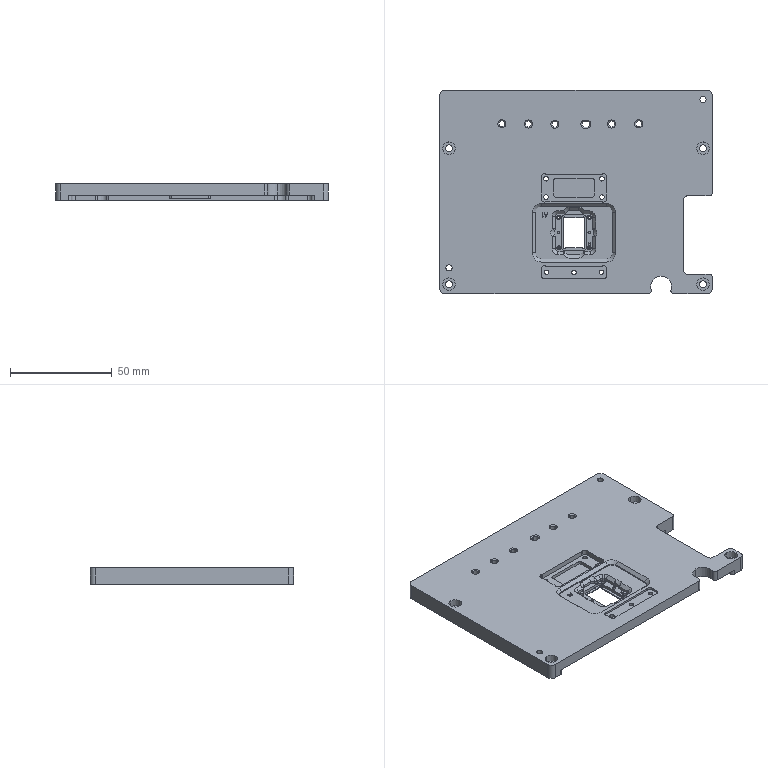NC program | NX | posted with a generic post | part box 134 x 100 x 8 mm
Lines 2719 to 3418 of 3418:
(CUTTERCOMP20 , TOOL : D1)
N5376 T20 M6
N5378 G54
N5380 G17 G0 G90 X0.695 Y-29.394 S9500 M3
N5382 G43 Z30. H20
N5384 Z-0.4
N5386 G94 G1 X0.839 Y-29.355 Z-0.408 F1000.
N5388 X1.143 Y-29.352 Z-0.424
N5390 X1.486 Y-29.45 Z-0.442
N5392 X1.783 Y-29.649 Z-0.461
N5394 X2.005 Y-29.928 Z-0.48
N5396 X2.119 Y-30.209 Z-0.496
N5398 X2.154 Y-30.578 Z-0.515
N5400 X2.07 Y-30.938 Z-0.535
N5402 X1.877 Y-31.254 Z-0.554
N5404 X1.594 Y-31.493 Z-0.573
N5406 X1.25 Y-31.629 Z-0.593
N5408 X1.049 Y-31.647 Z-0.603
N5410 X0.991 Z-0.606
N5412 X0.839 Y-31.645 Z-0.614
N5414 X0.441 Y-31.512 Z-0.636
N5416 X0.116 Y-31.246 Z-0.658
N5418 X-0.092 Y-30.881 Z-0.68
N5420 X-0.156 Y-30.466 Z-0.702
N5422 X-0.068 Y-30.056 Z-0.724
N5424 X0.084 Y-29.793 Z-0.74
N5426 X0.295 Y-29.583 Z-0.756
N5428 X0.552 Y-29.434 Z-0.771
N5430 X0.839 Y-29.355 Z-0.787
N5432 X1.143 Y-29.352 Z-0.803
N5434 X1.486 Y-29.45 Z-0.822
N5436 X1.783 Y-29.649 Z-0.84
N5438 X2.005 Y-29.928 Z-0.859
N5440 X2.119 Y-30.209 Z-0.875
N5442 X2.154 Y-30.578 Z-0.894
N5444 X2.07 Y-30.938 Z-0.914
N5446 X1.877 Y-31.254 Z-0.933
N5448 X1.594 Y-31.493 Z-0.953
N5450 X1.25 Y-31.629 Z-0.972
N5452 X1.098 Y-31.642 Z-0.98
N5454 G41 X1. Y-31.625 D20
N5456 X0.991
N5458 G2 X-0.125 Y-30.491 R1.125
N5460 X1. Y-31.625 R-1.125
N5462 G1 X0.928 Y-31.623 Z-0.981
N5464 X0.857 Y-31.616 Z-0.983
N5466 X0.786 Y-31.605 Z-0.984
N5468 X0.717 Y-31.589 Z-0.985
N5470 X0.648 Y-31.568 Z-0.986
N5472 X0.581 Y-31.544 Z-0.988
N5474 X0.515 Y-31.515 Z-0.989
N5476 X0.452 Y-31.482 Z-0.99
N5478 X0.39 Y-31.445 Z-0.991
N5480 X0.331 Y-31.405 Z-0.993
N5482 X0.275 Y-31.36 Z-0.994
N5484 X0.222 Y-31.313 Z-0.995
N5486 X0.172 Y-31.261 Z-0.996
N5488 X0.125 Y-31.207 Z-0.998
N5490 X0.082 Y-31.15 Z-0.999
N5492 X0.042 Y-31.09 Z-1.
N5494 X0.007 Y-31.028 Z-1.001
N5496 X-0.025 Y-30.964 Z-1.003
N5498 X-0.052 Y-30.898 Z-1.004
N5500 X-0.076 Y-30.83 Z-1.005
N5502 X-0.094 Y-30.761 Z-1.006
N5504 X-0.109 Y-30.691 Z-1.008
N5506 X-0.119 Y-30.62 Z-1.009
N5508 X-0.124 Y-30.548 Z-1.01
N5510 X-0.125 Y-30.477 Z-1.011
N5512 X-0.121 Y-30.405 Z-1.013
N5514 X-0.113 Y-30.334 Z-1.014
N5516 X-0.1 Y-30.264 Z-1.015
N5518 X-0.083 Y-30.194 Z-1.016
N5520 X-0.061 Y-30.126 Z-1.018
N5522 X-0.035 Y-30.059 Z-1.019
N5524 X-0.005 Y-29.994 Z-1.02
N5526 X0.029 Y-29.931 Z-1.021
N5528 X0.067 Y-29.871 Z-1.023
N5530 X0.109 Y-29.813 Z-1.024
N5532 X0.155 Y-29.758 Z-1.025
N5534 X0.204 Y-29.705 Z-1.026
N5536 X0.256 Y-29.656 Z-1.028
N5538 X0.311 Y-29.611 Z-1.029
N5540 X0.369 Y-29.569 Z-1.03
N5542 X0.43 Y-29.53 Z-1.031
N5544 X0.492 Y-29.496 Z-1.033
N5546 X0.557 Y-29.466 Z-1.034
N5548 X0.624 Y-29.44 Z-1.035
N5550 X0.692 Y-29.418 Z-1.036
N5552 X0.762 Y-29.401 Z-1.038
N5554 X0.832 Y-29.388 Z-1.039
N5556 X0.903 Y-29.379 Z-1.04
N5558 X0.975 Y-29.375 Z-1.041
N5560 X1.046 Y-29.376 Z-1.043
N5562 X1.118 Y-29.381 Z-1.044
N5564 X1.189 Y-29.391 Z-1.045
N5566 X1.259 Y-29.405 Z-1.046
N5568 X1.328 Y-29.424 Z-1.048
N5570 X1.396 Y-29.447 Z-1.049
N5572 X1.462 Y-29.474 Z-1.05
N5574 X1.526 Y-29.506 Z-1.051
N5576 X1.588 Y-29.541 Z-1.053
N5578 X1.648 Y-29.581 Z-1.054
N5580 X1.706 Y-29.623 Z-1.055
N5582 X1.76 Y-29.67 Z-1.056
N5584 X1.811 Y-29.72 Z-1.058
N5586 X1.859 Y-29.773 Z-1.059
N5588 X1.903 Y-29.83 Z-1.06
N5590 G2 X1. Y-31.625 R1.125
N5592 G1 X0.928 Y-31.623 Z-1.061
N5594 X0.857 Y-31.616 Z-1.063
N5596 X0.786 Y-31.605 Z-1.064
N5598 X0.717 Y-31.589 Z-1.065
N5600 X0.648 Y-31.568 Z-1.066
N5602 X0.581 Y-31.544 Z-1.068
N5604 X0.515 Y-31.515 Z-1.069
N5606 X0.452 Y-31.482 Z-1.07
N5608 X0.39 Y-31.445 Z-1.071
N5610 X0.331 Y-31.405 Z-1.073
N5612 X0.275 Y-31.36 Z-1.074
N5614 X0.222 Y-31.312 Z-1.075
N5616 X0.172 Y-31.261 Z-1.076
N5618 X0.125 Y-31.207 Z-1.078
N5620 X0.082 Y-31.15 Z-1.079
N5622 X0.042 Y-31.09 Z-1.08
N5624 X0.007 Y-31.028 Z-1.081
N5626 X-0.025 Y-30.964 Z-1.083
N5628 X-0.052 Y-30.898 Z-1.084
N5630 X-0.076 Y-30.83 Z-1.085
N5632 X-0.094 Y-30.761 Z-1.086
N5634 X-0.109 Y-30.691 Z-1.088
N5636 X-0.119 Y-30.62 Z-1.089
N5638 X-0.124 Y-30.548 Z-1.09
N5640 X-0.125 Y-30.477 Z-1.091
N5642 X-0.121 Y-30.405 Z-1.093
N5644 X-0.113 Y-30.334 Z-1.094
N5646 X-0.1 Y-30.264 Z-1.095
N5648 X-0.083 Y-30.194 Z-1.096
N5650 X-0.061 Y-30.126 Z-1.098
N5652 X-0.035 Y-30.059 Z-1.099
N5654 X-0.005 Y-29.994 Z-1.1
N5656 X0.029 Y-29.931 Z-1.101
N5658 X0.067 Y-29.871 Z-1.103
N5660 X0.109 Y-29.813 Z-1.104
N5662 X0.155 Y-29.758 Z-1.105
N5664 X0.204 Y-29.705 Z-1.106
N5666 X0.256 Y-29.656 Z-1.108
N5668 X0.311 Y-29.611 Z-1.109
N5670 X0.369 Y-29.569 Z-1.11
N5672 X0.43 Y-29.53 Z-1.111
N5674 X0.492 Y-29.496 Z-1.113
N5676 X0.557 Y-29.466 Z-1.114
N5678 X0.624 Y-29.439 Z-1.115
N5680 X0.692 Y-29.418 Z-1.116
N5682 X0.762 Y-29.401 Z-1.118
N5684 X0.832 Y-29.388 Z-1.119
N5686 X0.903 Y-29.379 Z-1.12
N5688 X0.975 Y-29.375 Z-1.121
N5690 X1.046 Y-29.376 Z-1.123
N5692 X1.118 Y-29.381 Z-1.124
N5694 X1.189 Y-29.391 Z-1.125
N5696 X1.259 Y-29.405 Z-1.126
N5698 X1.328 Y-29.424 Z-1.128
N5700 X1.396 Y-29.447 Z-1.129
N5702 X1.462 Y-29.474 Z-1.13
N5704 X1.526 Y-29.506 Z-1.131
N5706 X1.588 Y-29.541 Z-1.133
N5708 G2 X1. Y-31.625 R1.125
N5710 G1 X0.928 Y-31.623 Z-1.134
N5712 X0.857 Y-31.616 Z-1.135
N5714 X0.786 Y-31.605 Z-1.136
N5716 X0.717 Y-31.589 Z-1.138
N5718 X0.648 Y-31.569 Z-1.139
N5720 X0.581 Y-31.544 Z-1.14
N5722 X0.515 Y-31.515 Z-1.141
N5724 X0.452 Y-31.482 Z-1.143
N5726 X0.39 Y-31.445 Z-1.144
N5728 X0.331 Y-31.405 Z-1.145
N5730 X0.275 Y-31.36 Z-1.146
N5732 X0.222 Y-31.312 Z-1.148
N5734 X0.172 Y-31.261 Z-1.149
N5736 X0.125 Y-31.207 Z-1.15
N5738 X0.082 Y-31.15 Z-1.151
N5740 X0.042 Y-31.09 Z-1.153
N5742 X0.007 Y-31.028 Z-1.154
N5744 X-0.025 Y-30.964 Z-1.155
N5746 X-0.052 Y-30.898 Z-1.156
N5748 X-0.076 Y-30.83 Z-1.158
N5750 X-0.094 Y-30.761 Z-1.159
N5752 X-0.109 Y-30.691 Z-1.16
N5754 X-0.119 Y-30.62 Z-1.161
N5756 X-0.124 Y-30.548 Z-1.163
N5758 X-0.125 Y-30.477 Z-1.164
N5760 X-0.121 Y-30.405 Z-1.165
N5762 X-0.113 Y-30.334 Z-1.166
N5764 X-0.1 Y-30.264 Z-1.168
N5766 X-0.083 Y-30.194 Z-1.169
N5768 X-0.061 Y-30.126 Z-1.17
N5770 X-0.035 Y-30.059 Z-1.171
N5772 X-0.005 Y-29.994 Z-1.173
N5774 X0.029 Y-29.931 Z-1.174
N5776 X0.067 Y-29.871 Z-1.175
N5778 X0.109 Y-29.813 Z-1.176
N5780 X0.155 Y-29.758 Z-1.178
N5782 X0.204 Y-29.705 Z-1.179
N5784 X0.256 Y-29.656 Z-1.18
N5786 X0.311 Y-29.611 Z-1.181
N5788 X0.369 Y-29.568 Z-1.183
N5790 X0.43 Y-29.53 Z-1.184
N5792 X0.492 Y-29.496 Z-1.185
N5794 X0.557 Y-29.466 Z-1.186
N5796 X0.624 Y-29.439 Z-1.188
N5798 X0.692 Y-29.418 Z-1.189
N5800 X0.762 Y-29.401 Z-1.19
N5802 X0.832 Y-29.388 Z-1.191
N5804 X0.903 Y-29.379 Z-1.193
N5806 X0.975 Y-29.375 Z-1.194
N5808 X1.046 Y-29.376 Z-1.195
N5810 X1.118 Y-29.381 Z-1.196
N5812 X1.189 Y-29.391 Z-1.198
N5814 X1.259 Y-29.405 Z-1.199
N5816 X1.328 Y-29.424 Z-1.2
N5818 X1.396 Y-29.447 Z-1.201
N5820 X1.462 Y-29.474 Z-1.203
N5822 X1.526 Y-29.506 Z-1.204
N5824 X1.588 Y-29.541 Z-1.205
N5826 G2 X1. Y-31.625 R1.125
N5828 G1 X0.928 Y-31.623 Z-1.206
N5830 X0.857 Y-31.616 Z-1.208
N5832 X0.786 Y-31.605 Z-1.209
N5834 X0.717 Y-31.589 Z-1.21
N5836 X0.648 Y-31.569 Z-1.211
N5838 X0.581 Y-31.544 Z-1.213
N5840 X0.515 Y-31.515 Z-1.214
N5842 X0.452 Y-31.482 Z-1.215
N5844 X0.39 Y-31.445 Z-1.216
N5846 X0.331 Y-31.405 Z-1.218
N5848 X0.275 Y-31.36 Z-1.219
N5850 X0.222 Y-31.312 Z-1.22
N5852 X0.172 Y-31.261 Z-1.221
N5854 X0.125 Y-31.207 Z-1.223
N5856 X0.082 Y-31.15 Z-1.224
N5858 X0.042 Y-31.09 Z-1.225
N5860 X0.007 Y-31.028 Z-1.226
N5862 X-0.025 Y-30.964 Z-1.228
N5864 X-0.052 Y-30.898 Z-1.229
N5866 X-0.076 Y-30.83 Z-1.23
N5868 X-0.094 Y-30.761 Z-1.231
N5870 X-0.109 Y-30.691 Z-1.233
N5872 X-0.119 Y-30.62 Z-1.234
N5874 X-0.124 Y-30.548 Z-1.235
N5876 X-0.125 Y-30.477 Z-1.236
N5878 X-0.121 Y-30.405 Z-1.238
N5880 X-0.113 Y-30.334 Z-1.239
N5882 X-0.1 Y-30.264 Z-1.24
N5884 X-0.083 Y-30.194 Z-1.241
N5886 X-0.061 Y-30.126 Z-1.243
N5888 X-0.035 Y-30.059 Z-1.244
N5890 X-0.005 Y-29.994 Z-1.245
N5892 X0.029 Y-29.931 Z-1.246
N5894 X0.067 Y-29.871 Z-1.248
N5896 X0.109 Y-29.813 Z-1.249
N5898 X0.155 Y-29.758 Z-1.25
N5900 X0.204 Y-29.705 Z-1.251
N5902 X0.256 Y-29.656 Z-1.253
N5904 X0.311 Y-29.611 Z-1.254
N5906 X0.369 Y-29.568 Z-1.255
N5908 X0.43 Y-29.53 Z-1.256
N5910 X0.492 Y-29.496 Z-1.258
N5912 X0.557 Y-29.466 Z-1.259
N5914 X0.624 Y-29.439 Z-1.26
N5916 X0.692 Y-29.418 Z-1.261
N5918 X0.762 Y-29.401 Z-1.263
N5920 X0.832 Y-29.388 Z-1.264
N5922 X0.903 Y-29.379 Z-1.265
N5924 X0.975 Y-29.375 Z-1.266
N5926 X1.046 Y-29.376 Z-1.268
N5928 X1.118 Y-29.381 Z-1.269
N5930 X1.189 Y-29.391 Z-1.27
N5932 X1.259 Y-29.405 Z-1.271
N5934 X1.328 Y-29.424 Z-1.273
N5936 X1.396 Y-29.447 Z-1.274
N5938 X1.462 Y-29.474 Z-1.275
N5940 X1.526 Y-29.506 Z-1.276
N5942 X1.588 Y-29.541 Z-1.278
N5944 G2 X1. Y-31.625 R1.125
N5946 G1 X0.928 Y-31.623 Z-1.279
N5948 X0.857 Y-31.616 Z-1.28
N5950 X0.786 Y-31.605 Z-1.281
N5952 X0.717 Y-31.589 Z-1.283
N5954 X0.648 Y-31.568 Z-1.284
N5956 X0.581 Y-31.544 Z-1.285
N5958 X0.515 Y-31.515 Z-1.286
N5960 X0.452 Y-31.482 Z-1.288
N5962 X0.39 Y-31.445 Z-1.289
N5964 X0.331 Y-31.405 Z-1.29
N5966 X0.275 Y-31.36 Z-1.291
N5968 X0.222 Y-31.312 Z-1.293
N5970 X0.172 Y-31.261 Z-1.294
N5972 X0.125 Y-31.207 Z-1.295
N5974 X0.082 Y-31.15 Z-1.296
N5976 X0.042 Y-31.09 Z-1.298
N5978 X0.007 Y-31.028 Z-1.299
N5980 X-0.025 Y-30.964 Z-1.3
N5982 X-0.052 Y-30.898 Z-1.301
N5984 X-0.076 Y-30.83 Z-1.303
N5986 X-0.094 Y-30.761 Z-1.304
N5988 X-0.109 Y-30.691 Z-1.305
N5990 X-0.119 Y-30.62 Z-1.306
N5992 X-0.124 Y-30.548 Z-1.308
N5994 X-0.125 Y-30.477 Z-1.309
N5996 X-0.121 Y-30.405 Z-1.31
N5998 X-0.113 Y-30.334 Z-1.311
N6000 X-0.1 Y-30.264 Z-1.313
N6002 X-0.083 Y-30.194 Z-1.314
N6004 X-0.061 Y-30.126 Z-1.315
N6006 X-0.035 Y-30.059 Z-1.316
N6008 X-0.005 Y-29.994 Z-1.318
N6010 X0.029 Y-29.931 Z-1.319
N6012 X0.067 Y-29.871 Z-1.32
N6014 X0.109 Y-29.813 Z-1.321
N6016 X0.155 Y-29.758 Z-1.323
N6018 X0.204 Y-29.705 Z-1.324
N6020 X0.256 Y-29.656 Z-1.325
N6022 X0.311 Y-29.611 Z-1.326
N6024 X0.369 Y-29.569 Z-1.328
N6026 X0.43 Y-29.53 Z-1.329
N6028 X0.492 Y-29.496 Z-1.33
N6030 X0.557 Y-29.466 Z-1.331
N6032 X0.624 Y-29.439 Z-1.333
N6034 X0.692 Y-29.418 Z-1.334
N6036 X0.762 Y-29.401 Z-1.335
N6038 X0.832 Y-29.388 Z-1.336
N6040 X0.903 Y-29.379 Z-1.338
N6042 X0.975 Y-29.375 Z-1.339
N6044 X1.046 Y-29.376 Z-1.34
N6046 X1.118 Y-29.381 Z-1.341
N6048 X1.189 Y-29.391 Z-1.343
N6050 X1.259 Y-29.405 Z-1.344
N6052 X1.328 Y-29.424 Z-1.345
N6054 X1.396 Y-29.447 Z-1.346
N6056 X1.462 Y-29.474 Z-1.348
N6058 X1.526 Y-29.506 Z-1.349
N6060 X1.588 Y-29.541 Z-1.35
N6062 G2 X1.959 Y-31.088 R1.125
N6064 X1.588 Y-29.541 R-1.125
N6066 G40
N6068 G1 X1.681 Y-29.578
N6070 Z-0.85
N6072 G0 Z30.
N6074 X0.695 Y-8.394
N6076 Z-0.4
N6078 G1 X0.839 Y-8.355 Z-0.408
N6080 X1.143 Y-8.352 Z-0.424
N6082 X1.486 Y-8.45 Z-0.442
N6084 X1.783 Y-8.649 Z-0.461
N6086 X2.005 Y-8.928 Z-0.48
N6088 X2.119 Y-9.209 Z-0.496
N6090 X2.154 Y-9.578 Z-0.515
N6092 X2.07 Y-9.938 Z-0.535
N6094 X1.877 Y-10.254 Z-0.554
N6096 X1.594 Y-10.493 Z-0.573
N6098 X1.25 Y-10.629 Z-0.593
N6100 X1.049 Y-10.647 Z-0.603
N6102 X0.991 Z-0.606
N6104 X0.839 Y-10.645 Z-0.614
N6106 X0.441 Y-10.512 Z-0.636
N6108 X0.116 Y-10.246 Z-0.658
N6110 X-0.092 Y-9.881 Z-0.68
N6112 X-0.156 Y-9.466 Z-0.702
N6114 X-0.068 Y-9.056 Z-0.724
N6116 X0.084 Y-8.793 Z-0.74
N6118 X0.295 Y-8.583 Z-0.756
N6120 X0.552 Y-8.434 Z-0.771
N6122 X0.839 Y-8.355 Z-0.787
N6124 X1.143 Y-8.352 Z-0.803
N6126 X1.486 Y-8.45 Z-0.822
N6128 X1.783 Y-8.649 Z-0.84
N6130 X2.005 Y-8.928 Z-0.859
N6132 X2.119 Y-9.209 Z-0.875
N6134 X2.154 Y-9.578 Z-0.894
N6136 X2.07 Y-9.938 Z-0.914
N6138 X1.877 Y-10.254 Z-0.933
N6140 X1.594 Y-10.493 Z-0.953
N6142 X1.25 Y-10.629 Z-0.972
N6144 X1.098 Y-10.642 Z-0.98
N6146 G41 X1. Y-10.625
N6148 X0.991
N6150 G2 X-0.125 Y-9.491 R1.125
N6152 X1. Y-10.625 R-1.125
N6154 G1 X0.928 Y-10.623 Z-0.981
N6156 X0.857 Y-10.616 Z-0.983
N6158 X0.786 Y-10.605 Z-0.984
N6160 X0.717 Y-10.589 Z-0.985
N6162 X0.648 Y-10.568 Z-0.986
N6164 X0.581 Y-10.544 Z-0.988
N6166 X0.515 Y-10.515 Z-0.989
N6168 X0.452 Y-10.482 Z-0.99
N6170 X0.39 Y-10.445 Z-0.991
N6172 X0.331 Y-10.405 Z-0.993
N6174 X0.275 Y-10.36 Z-0.994
N6176 X0.222 Y-10.313 Z-0.995
N6178 X0.172 Y-10.261 Z-0.996
N6180 X0.125 Y-10.207 Z-0.998
N6182 X0.082 Y-10.15 Z-0.999
N6184 X0.042 Y-10.09 Z-1.
N6186 X0.007 Y-10.028 Z-1.001
N6188 X-0.025 Y-9.964 Z-1.003
N6190 X-0.052 Y-9.898 Z-1.004
N6192 X-0.076 Y-9.83 Z-1.005
N6194 X-0.094 Y-9.761 Z-1.006
N6196 X-0.109 Y-9.691 Z-1.008
N6198 X-0.119 Y-9.62 Z-1.009
N6200 X-0.124 Y-9.548 Z-1.01
N6202 X-0.125 Y-9.477 Z-1.011
N6204 X-0.121 Y-9.405 Z-1.013
N6206 X-0.113 Y-9.334 Z-1.014
N6208 X-0.1 Y-9.264 Z-1.015
N6210 X-0.083 Y-9.194 Z-1.016
N6212 X-0.061 Y-9.126 Z-1.018
N6214 X-0.035 Y-9.059 Z-1.019
N6216 X-0.005 Y-8.994 Z-1.02
N6218 X0.029 Y-8.931 Z-1.021
N6220 X0.067 Y-8.871 Z-1.023
N6222 X0.109 Y-8.813 Z-1.024
N6224 X0.155 Y-8.758 Z-1.025
N6226 X0.204 Y-8.705 Z-1.026
N6228 X0.256 Y-8.656 Z-1.028
N6230 X0.311 Y-8.611 Z-1.029
N6232 X0.369 Y-8.569 Z-1.03
N6234 X0.43 Y-8.53 Z-1.031
N6236 X0.492 Y-8.496 Z-1.033
N6238 X0.557 Y-8.466 Z-1.034
N6240 X0.624 Y-8.44 Z-1.035
N6242 X0.692 Y-8.418 Z-1.036
N6244 X0.762 Y-8.401 Z-1.038
N6246 X0.832 Y-8.388 Z-1.039
N6248 X0.903 Y-8.379 Z-1.04
N6250 X0.975 Y-8.375 Z-1.041
N6252 X1.046 Y-8.376 Z-1.043
N6254 X1.118 Y-8.381 Z-1.044
N6256 X1.189 Y-8.391 Z-1.045
N6258 X1.259 Y-8.405 Z-1.046
N6260 X1.328 Y-8.424 Z-1.048
N6262 X1.396 Y-8.447 Z-1.049
N6264 X1.462 Y-8.474 Z-1.05
N6266 X1.526 Y-8.506 Z-1.051
N6268 X1.588 Y-8.541 Z-1.053
N6270 X1.648 Y-8.581 Z-1.054
N6272 X1.705 Y-8.624 Z-1.055
N6274 X1.76 Y-8.67 Z-1.056
N6276 X1.811 Y-8.72 Z-1.058
N6278 X1.859 Y-8.773 Z-1.059
N6280 X1.903 Y-8.83 Z-1.06
N6282 G2 X1. Y-10.625 R1.125
N6284 G1 X0.928 Y-10.623 Z-1.061
N6286 X0.857 Y-10.616 Z-1.063
N6288 X0.786 Y-10.605 Z-1.064
N6290 X0.717 Y-10.589 Z-1.065
N6292 X0.648 Y-10.568 Z-1.066
N6294 X0.581 Y-10.544 Z-1.068
N6296 X0.515 Y-10.515 Z-1.069
N6298 X0.452 Y-10.482 Z-1.07
N6300 X0.39 Y-10.445 Z-1.071
N6302 X0.331 Y-10.405 Z-1.073
N6304 X0.275 Y-10.36 Z-1.074
N6306 X0.222 Y-10.312 Z-1.075
N6308 X0.172 Y-10.261 Z-1.076
N6310 X0.125 Y-10.207 Z-1.078
N6312 X0.082 Y-10.15 Z-1.079
N6314 X0.042 Y-10.09 Z-1.08
N6316 X0.007 Y-10.028 Z-1.081
N6318 X-0.025 Y-9.964 Z-1.083
N6320 X-0.052 Y-9.898 Z-1.084
N6322 X-0.076 Y-9.83 Z-1.085
N6324 X-0.094 Y-9.761 Z-1.086
N6326 X-0.109 Y-9.691 Z-1.088
N6328 X-0.119 Y-9.62 Z-1.089
N6330 X-0.124 Y-9.548 Z-1.09
N6332 X-0.125 Y-9.477 Z-1.091
N6334 X-0.121 Y-9.405 Z-1.093
N6336 X-0.113 Y-9.334 Z-1.094
N6338 X-0.1 Y-9.264 Z-1.095
N6340 X-0.083 Y-9.194 Z-1.096
N6342 X-0.061 Y-9.126 Z-1.098
N6344 X-0.035 Y-9.059 Z-1.099
N6346 X-0.005 Y-8.994 Z-1.1
N6348 X0.029 Y-8.931 Z-1.101
N6350 X0.067 Y-8.871 Z-1.103
N6352 X0.109 Y-8.813 Z-1.104
N6354 X0.155 Y-8.758 Z-1.105
N6356 X0.204 Y-8.705 Z-1.106
N6358 X0.256 Y-8.656 Z-1.108
N6360 X0.311 Y-8.611 Z-1.109
N6362 X0.369 Y-8.569 Z-1.11
N6364 X0.43 Y-8.53 Z-1.111
N6366 X0.492 Y-8.496 Z-1.113
N6368 X0.557 Y-8.466 Z-1.114
N6370 X0.624 Y-8.44 Z-1.115
N6372 X0.692 Y-8.418 Z-1.116
N6374 X0.762 Y-8.401 Z-1.118
N6376 X0.832 Y-8.388 Z-1.119
N6378 X0.903 Y-8.379 Z-1.12
N6380 X0.975 Y-8.375 Z-1.121
N6382 X1.046 Y-8.376 Z-1.123
N6384 X1.118 Y-8.381 Z-1.124
N6386 X1.189 Y-8.391 Z-1.125
N6388 X1.259 Y-8.405 Z-1.126
N6390 X1.328 Y-8.424 Z-1.128
N6392 X1.396 Y-8.447 Z-1.129
N6394 X1.462 Y-8.474 Z-1.13
N6396 X1.526 Y-8.506 Z-1.131
N6398 X1.588 Y-8.541 Z-1.133
N6400 G2 X1. Y-10.625 R1.125
N6402 G1 X0.928 Y-10.623 Z-1.134
N6404 X0.857 Y-10.616 Z-1.135
N6406 X0.786 Y-10.605 Z-1.136
N6408 X0.717 Y-10.589 Z-1.138
N6410 X0.648 Y-10.568 Z-1.139
N6412 X0.581 Y-10.544 Z-1.14
N6414 X0.515 Y-10.515 Z-1.141
N6416 X0.452 Y-10.482 Z-1.143
N6418 X0.39 Y-10.445 Z-1.144
N6420 X0.331 Y-10.405 Z-1.145
N6422 X0.275 Y-10.36 Z-1.146
N6424 X0.222 Y-10.312 Z-1.148
N6426 X0.172 Y-10.261 Z-1.149
N6428 X0.125 Y-10.207 Z-1.15
N6430 X0.082 Y-10.15 Z-1.151
N6432 X0.042 Y-10.09 Z-1.153
N6434 X0.007 Y-10.028 Z-1.154
N6436 X-0.025 Y-9.964 Z-1.155
N6438 X-0.052 Y-9.898 Z-1.156
N6440 X-0.076 Y-9.83 Z-1.158
N6442 X-0.094 Y-9.761 Z-1.159
N6444 X-0.109 Y-9.691 Z-1.16
N6446 X-0.119 Y-9.62 Z-1.161
N6448 X-0.124 Y-9.548 Z-1.163
N6450 X-0.125 Y-9.477 Z-1.164
N6452 X-0.121 Y-9.405 Z-1.165
N6454 X-0.113 Y-9.334 Z-1.166
N6456 X-0.1 Y-9.264 Z-1.168
N6458 X-0.083 Y-9.194 Z-1.169
N6460 X-0.061 Y-9.126 Z-1.17
N6462 X-0.035 Y-9.059 Z-1.171
N6464 X-0.005 Y-8.994 Z-1.173
N6466 X0.029 Y-8.931 Z-1.174
N6468 X0.067 Y-8.871 Z-1.175
N6470 X0.109 Y-8.813 Z-1.176
N6472 X0.155 Y-8.758 Z-1.178
N6474 X0.204 Y-8.705 Z-1.179
N6476 X0.256 Y-8.656 Z-1.18
N6478 X0.311 Y-8.611 Z-1.181
N6480 X0.369 Y-8.569 Z-1.183
N6482 X0.43 Y-8.53 Z-1.184
N6484 X0.492 Y-8.496 Z-1.185
N6486 X0.557 Y-8.466 Z-1.186
N6488 X0.624 Y-8.44 Z-1.188
N6490 X0.692 Y-8.418 Z-1.189
N6492 X0.762 Y-8.401 Z-1.19
N6494 X0.832 Y-8.388 Z-1.191
N6496 X0.903 Y-8.379 Z-1.193
N6498 X0.975 Y-8.375 Z-1.194
N6500 X1.046 Y-8.376 Z-1.195
N6502 X1.118 Y-8.381 Z-1.196
N6504 X1.189 Y-8.391 Z-1.198
N6506 X1.259 Y-8.405 Z-1.199
N6508 X1.328 Y-8.424 Z-1.2
N6510 X1.396 Y-8.447 Z-1.201
N6512 X1.462 Y-8.474 Z-1.203
N6514 X1.526 Y-8.506 Z-1.204
N6516 X1.588 Y-8.541 Z-1.205
N6518 G2 X1. Y-10.625 R1.125
N6520 G1 X0.928 Y-10.623 Z-1.206
N6522 X0.857 Y-10.616 Z-1.208
N6524 X0.786 Y-10.605 Z-1.209
N6526 X0.717 Y-10.589 Z-1.21
N6528 X0.648 Y-10.568 Z-1.211
N6530 X0.581 Y-10.544 Z-1.213
N6532 X0.515 Y-10.515 Z-1.214
N6534 X0.452 Y-10.482 Z-1.215
N6536 X0.39 Y-10.445 Z-1.216
N6538 X0.331 Y-10.405 Z-1.218
N6540 X0.275 Y-10.36 Z-1.219
N6542 X0.222 Y-10.312 Z-1.22
N6544 X0.172 Y-10.261 Z-1.221
N6546 X0.125 Y-10.207 Z-1.223
N6548 X0.082 Y-10.15 Z-1.224
N6550 X0.042 Y-10.09 Z-1.225
N6552 X0.007 Y-10.028 Z-1.226
N6554 X-0.025 Y-9.964 Z-1.228
N6556 X-0.052 Y-9.898 Z-1.229
N6558 X-0.076 Y-9.83 Z-1.23
N6560 X-0.094 Y-9.761 Z-1.231
N6562 X-0.109 Y-9.691 Z-1.233
N6564 X-0.119 Y-9.62 Z-1.234
N6566 X-0.124 Y-9.548 Z-1.235
N6568 X-0.125 Y-9.477 Z-1.236
N6570 X-0.121 Y-9.405 Z-1.238
N6572 X-0.113 Y-9.334 Z-1.239
N6574 X-0.1 Y-9.264 Z-1.24
N6576 X-0.083 Y-9.194 Z-1.241
N6578 X-0.061 Y-9.126 Z-1.243
N6580 X-0.035 Y-9.059 Z-1.244
N6582 X-0.005 Y-8.994 Z-1.245
N6584 X0.029 Y-8.931 Z-1.246
N6586 X0.067 Y-8.871 Z-1.248
N6588 X0.109 Y-8.813 Z-1.249
N6590 X0.155 Y-8.758 Z-1.25
N6592 X0.204 Y-8.705 Z-1.251
N6594 X0.256 Y-8.656 Z-1.253
N6596 X0.311 Y-8.611 Z-1.254
N6598 X0.369 Y-8.569 Z-1.255
N6600 X0.43 Y-8.53 Z-1.256
N6602 X0.492 Y-8.496 Z-1.258
N6604 X0.557 Y-8.466 Z-1.259
N6606 X0.624 Y-8.44 Z-1.26
N6608 X0.692 Y-8.418 Z-1.261
N6610 X0.762 Y-8.401 Z-1.263
N6612 X0.832 Y-8.388 Z-1.264
N6614 X0.903 Y-8.379 Z-1.265
N6616 X0.975 Y-8.375 Z-1.266
N6618 X1.046 Y-8.376 Z-1.268
N6620 X1.118 Y-8.381 Z-1.269
N6622 X1.189 Y-8.391 Z-1.27
N6624 X1.259 Y-8.405 Z-1.271
N6626 X1.328 Y-8.424 Z-1.273
N6628 X1.396 Y-8.447 Z-1.274
N6630 X1.462 Y-8.474 Z-1.275
N6632 X1.526 Y-8.506 Z-1.276
N6634 X1.588 Y-8.541 Z-1.278
N6636 G2 X1. Y-10.625 R1.125
N6638 G1 X0.928 Y-10.623 Z-1.279
N6640 X0.857 Y-10.616 Z-1.28
N6642 X0.786 Y-10.605 Z-1.281
N6644 X0.717 Y-10.589 Z-1.283
N6646 X0.648 Y-10.568 Z-1.284
N6648 X0.581 Y-10.544 Z-1.285
N6650 X0.515 Y-10.515 Z-1.286
N6652 X0.452 Y-10.482 Z-1.288
N6654 X0.39 Y-10.445 Z-1.289
N6656 X0.331 Y-10.405 Z-1.29
N6658 X0.275 Y-10.36 Z-1.291
N6660 X0.222 Y-10.312 Z-1.293
N6662 X0.172 Y-10.261 Z-1.294
N6664 X0.125 Y-10.207 Z-1.295
N6666 X0.082 Y-10.15 Z-1.296
N6668 X0.042 Y-10.09 Z-1.298
N6670 X0.007 Y-10.028 Z-1.299
N6672 X-0.025 Y-9.964 Z-1.3
N6674 X-0.052 Y-9.898 Z-1.301
N6676 X-0.076 Y-9.83 Z-1.303
N6678 X-0.094 Y-9.761 Z-1.304
N6680 X-0.109 Y-9.691 Z-1.305
N6682 X-0.119 Y-9.62 Z-1.306
N6684 X-0.124 Y-9.548 Z-1.308
N6686 X-0.125 Y-9.477 Z-1.309
N6688 X-0.121 Y-9.405 Z-1.31
N6690 X-0.113 Y-9.334 Z-1.311
N6692 X-0.1 Y-9.264 Z-1.313
N6694 X-0.083 Y-9.194 Z-1.314
N6696 X-0.061 Y-9.126 Z-1.315
N6698 X-0.035 Y-9.059 Z-1.316
N6700 X-0.005 Y-8.994 Z-1.318
N6702 X0.029 Y-8.931 Z-1.319
N6704 X0.067 Y-8.871 Z-1.32
N6706 X0.109 Y-8.813 Z-1.321
N6708 X0.155 Y-8.758 Z-1.323
N6710 X0.204 Y-8.705 Z-1.324
N6712 X0.256 Y-8.656 Z-1.325
N6714 X0.311 Y-8.611 Z-1.326
N6716 X0.369 Y-8.569 Z-1.328
N6718 X0.43 Y-8.53 Z-1.329
N6720 X0.492 Y-8.496 Z-1.33
N6722 X0.557 Y-8.466 Z-1.331
N6724 X0.624 Y-8.44 Z-1.333
N6726 X0.692 Y-8.418 Z-1.334
N6728 X0.762 Y-8.401 Z-1.335
N6730 X0.832 Y-8.388 Z-1.336
N6732 X0.903 Y-8.379 Z-1.338
N6734 X0.975 Y-8.375 Z-1.339
N6736 X1.046 Y-8.376 Z-1.34
N6738 X1.118 Y-8.381 Z-1.341
N6740 X1.189 Y-8.391 Z-1.343
N6742 X1.259 Y-8.405 Z-1.344
N6744 X1.328 Y-8.424 Z-1.345
N6746 X1.396 Y-8.447 Z-1.346
N6748 X1.462 Y-8.474 Z-1.348
N6750 X1.526 Y-8.506 Z-1.349
N6752 X1.588 Y-8.541 Z-1.35
N6754 G2 X1.959 Y-10.088 R1.125
N6756 X1.588 Y-8.541 R-1.125
N6758 G40
N6760 G1 X1.681 Y-8.578
N6762 Z-0.85
N6764 G0 Z30.
N6766 M5
N6768 M2